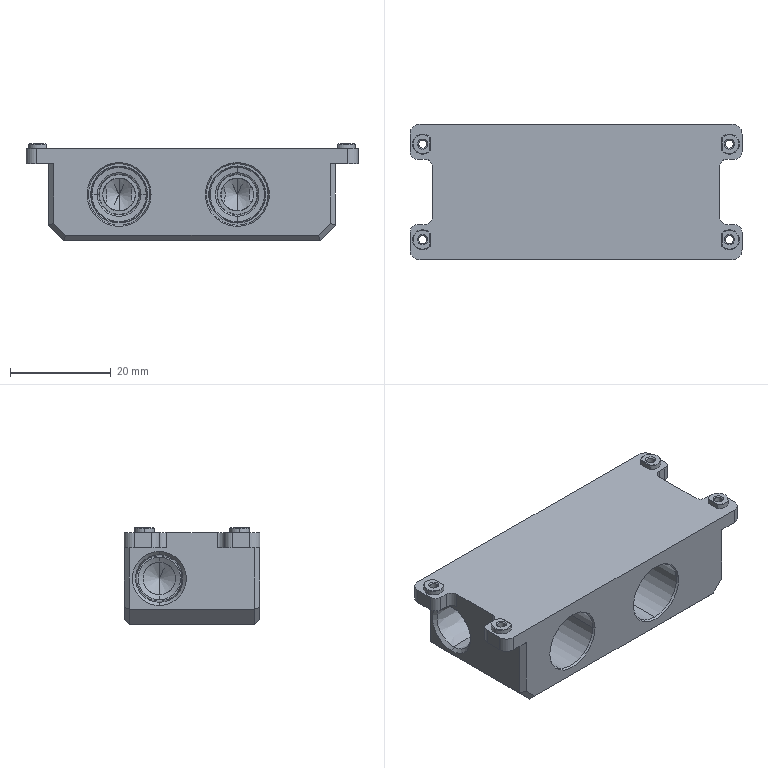NC program | NX | posted with a generic post | part box 66 x 27 x 19.25 mm
Lines 1 to 1685 of 6448, first 1517 of 1665 lines:
N10 G17 G21 G94 G90
(FLOOR_WALL , TOOL : D50面刀)
N12 T01 M6
N14 G53
N16 G17 G0 G90 X7.5 Y-69.5 S4500 M3
N18 G43 Z20. H1
N20 Z2.
N22 G94 G1 Z0. F800.
N24 Y-65.5
N26 Y65.5
N28 Y69.5
N30 Z2.
N32 G0 Z20.
N34 M5
(ADAPTIVE_MILLING , TOOL : D8开粗)
N36 T02 M6
N38 G53
N40 G17 G0 G90 X-7.067 Y-44.53 S7500 M3
N42 G43 Z20. H2
N44 Z-17.
N46 G94 G1 X-7.079 Y-44.38 Z-17.937 F2500.
N48 X-7.092 Y-44.231 Z-18.308
N50 X-7.105 Y-44.081 Z-18.58
N52 X-7.118 Y-43.932 Z-18.8
N54 X-7.131 Y-43.783 Z-18.984
N56 X-7.143 Y-43.633 Z-19.142
N58 X-7.156 Y-43.484 Z-19.28
N60 X-7.169 Y-43.334 Z-19.4
N62 X-7.182 Y-43.185 Z-19.505
N64 X-7.195 Y-43.035 Z-19.598
N66 X-7.207 Y-42.886 Z-19.679
N68 X-7.22 Y-42.736 Z-19.75
N70 X-7.233 Y-42.587 Z-19.81
N72 X-7.246 Y-42.437 Z-19.862
N74 X-7.259 Y-42.288 Z-19.905
N76 X-7.271 Y-42.139 Z-19.939
N78 X-7.284 Y-41.989 Z-19.966
N80 X-7.297 Y-41.84 Z-19.985
N82 X-7.31 Y-41.69 Z-19.996
N84 X-7.323 Y-41.541 Z-20.
N86 X-7.439 Y-40.185
N88 G3 X-7.858 Y-39.545 R0.809
N90 X-10.395 Y-38.825 R6.931
N92 X-13.916 Y-38.561 R62.132
N94 G2 X-16.854 Y-36.642 R4.621
N96 X-18.414 Y-32.843 R9.486
N98 X-18.931 Y-27.022 R34.366
N100 X-18.998 Y-14.123 R739.978
N102 G1 Y33.002
N104 G2 X-17.593 Y35.893 R4.169
N106 X-13.951 Y37.753 R8.174
N108 X-8.674 Y38.391 R25.798
N110 X4.375 Y38.498 R405.868
N112 G1 X13.774 Y38.484
N114 G2 X16.724 Y36.727 R4.45
N116 X18.401 Y32.833 R9.165
N118 X18.921 Y27.315 R32.513
N120 X18.998 Y13.965 R618.083
N122 G1 X18.996 Y-33.074
N124 G2 X17.436 Y-36.046 R4.252
N126 X13.741 Y-37.808 R8.515
N128 X8.383 Y-38.403 R27.886
N130 X-5.191 Y-38.477 R389.585
N132 X-9.5 Y-37.957 R98.771
N134 X-11.876 Y-37.672 R26.648
N136 X-14.578 Y-36.238 R6.14
N138 G1 X-14.89 Y-36.071
N140 X-15.814 Y-35.312
N142 X-16.573 Y-34.388
N144 X-17.136 Y-33.333
N146 X-17.483 Y-32.189
N148 G2 X-17.971 Y-22.311 R90.901
N150 G1 X-17.998 Y-11.361
N152 X-17.995 Y30.451
N154 G2 X-17.182 Y33.181 R5.655
N156 G1 X-17.135 Y33.336
N158 X-16.571 Y34.39
N160 X-15.812 Y35.314
N162 X-14.888 Y36.073
N164 X-13.833 Y36.636
N166 X-12.689 Y36.983
N168 G2 X-3.186 Y37.47 R89.967
N170 X11.198 Y37.482 R854.468
N172 X13.687 Y36.68 R5.673
N174 G1 X13.836 Y36.635
N176 X14.89 Y36.071
N178 X15.814 Y35.312
N180 X16.573 Y34.388
N182 X17.136 Y33.333
N184 X17.483 Y32.189
N186 G2 X17.973 Y22.011 R93.894
N188 G1 X17.998 Y11.211
N190 X17.994 Y-30.473
N192 G2 X17.181 Y-33.183 R5.661
N194 G1 X17.135 Y-33.336
N196 X16.571 Y-34.39
N198 X15.812 Y-35.314
N200 X14.888 Y-36.073
N202 X13.833 Y-36.636
N204 X12.689 Y-36.983
N206 G2 X3.186 Y-37.47 R89.76
N208 X-4.013 Y-37.453 R161.594
N210 X-8.025 Y-37.1 R101.274
N212 G1 X-11.501
N214 X-12.691 Y-36.982
N216 X-13.836 Y-36.635
N218 X-14.89 Y-36.071
N220 X-15.814 Y-35.312
N222 X-16.573 Y-34.388
N224 X-17.136 Y-33.333
N226 X-17.483 Y-32.189
N228 X-17.6 Y-30.999
N230 Y31.001
N232 X-17.482 Y32.191
N234 X-17.135 Y33.336
N236 X-16.571 Y34.39
N238 X-15.812 Y35.314
N240 X-14.888 Y36.073
N242 X-13.833 Y36.636
N244 X-12.689 Y36.983
N246 X-11.499 Y37.1
N248 X-7.999
N250 G2 X-6.217 Y36.844 R10.21
N252 G3 X-0.835 Y36.531 R41.818
N254 X5.498 Y36.515 R159.228
N256 X6.014 Y36.736 R3.667
N258 G2 X8.001 Y37.1 R6.513
N260 G1 X11.501
N262 X12.691 Y36.982
N264 X13.696 Y36.677
N266 X12.691 Y36.982
N268 X11.501 Y37.1
N270 X8.001
N272 G3 X6.014 Y36.736 R6.511
N274 G2 X3.976 Y36.143 R4.98
N276 X-4.811 Y36.15 R48.551
N278 G1 X-6.012 Y36.735
N280 X-6.806 Y36.957
N282 G2 X-4.63 Y35.963 R5.64
N284 G3 X-1.794 Y35.249 R8.388
N286 X3.699 Y35.265 R22.919
N288 X4.286 Y35.691 R1.168
N290 G1 X5.103 Y36.292
N292 X5.507 Y36.489
N294 G3 X3.925 Y35.315 R4.978
N296 G2 X1.942 Y34.752 R4.985
N298 X-3.594 Y35.122 R14.488
N300 X-4.284 Y35.689 R1.743
N302 G1 X-4.767 Y36.045
N304 G2 X-3.673 Y35.039 R5.141
N306 G3 X-1.437 Y34.121 R5.114
N308 X2.909 Y34.214 R9.441
N310 X3.306 Y34.511 R1.102
N312 G2 X4.002 Y35.389 R3.398
N314 G3 X3.178 Y34.325 R4.895
N316 G2 X1.424 Y33.644 R3.476
N318 X-3.021 Y34.236 R7.576
N320 X-3.589 Y34.95 R2.111
N322 G1 X-3.692 Y35.059
N324 G2 X-3.111 Y34.21 R6.402
N326 G3 X-1.161 Y33.134 R3.673
N328 X2.458 Y33.297 R5.928
N330 X2.879 Y33.709 R0.968
N332 G2 X3.244 Y34.415 R2.657
N334 G3 X2.787 Y33.504 R4.138
N336 G2 X1.45 Y32.767 R2.46
N338 X-2.649 Y33.424 R5.234
N340 X-3.039 Y34.098 R1.424
N342 G1 X-3.121 Y34.224
N344 G2 X-2.766 Y33.438 R5.334
N346 G3 X-1.68 Y32.604 R1.715
N348 G1 X1.779 Y32.612
N350 G3 X2.673 Y33.211 R1.013
N352 G1 X2.845 Y33.627
N354 G2 X2.348 Y32.776 R1.859
N356 X1.647 Y32.6 R1.117
N358 G1 X-1.872 Y32.608
N360 G2 X-2.786 Y33.487 R1.175
N362 G3 X-2.191 Y32.685 R1.281
N364 X-1.83 Y32.603 R3.588
N366 X-1.039 Y33.062 R0.801
N368 G1 X-0.792 Y33.804 Z-19.95
N370 X-0.559 Y34.551 Z-19.9
N372 X-0.43 Y34.968 F15000.
N374 X-0.287 Y35.38
N376 X-0.193 Y35.527
N378 X-0.07 Y35.652
N380 X0.729 Y36.296
N382 X1.535 Y36.931
N384 G2 X4.369 Y38.638 R15.893
N386 X6.671 Y39.42 R13.606
N388 X10.502 Y39.697 R10.132
N390 G1 X11.781 Y39.548
N392 X13.059 Y39.38
N394 G2 X18.414 Y35.931 R8.207
N396 G1 X20.089 Y33.489
N398 G2 X19.686 Y32.278 R0.8
N400 G1 X19.467 Y32.204
N402 X18.066 Y31.726 Z-19.995 F2500.
N404 X17.992 Y31.687 Z-20.
N406 G3 X17.6 Y30.999 R0.801
N408 G1 Y-31.001
N410 X17.482 Y-32.191
N412 X17.135 Y-33.336
N414 X16.571 Y-34.39
N416 X15.812 Y-35.314
N418 X14.888 Y-36.073
N420 X13.833 Y-36.636
N422 X12.689 Y-36.983
N424 X11.5 Y-37.1
N426 X7.999
N428 G2 X6.234 Y-36.847 R9.97
N430 G3 X0.564 Y-36.526 R42.919
N432 G2 X-5.051 Y-36.337 R88.056
N434 G1 X-5.321 Y-36.398
N436 G2 X-6.991 Y-37.008 R6.001
N438 G1 X-8.076 Y-37.1
N440 G3 X-5.186 Y-36.333 R5.83
N442 G2 X-2.94 Y-36.014 R8.254
N444 X4.756 Y-36.137 R58.568
N446 X5.1 Y-36.291 R1.779
N448 G3 X6.806 Y-36.957 R6.106
N450 G2 X4.741 Y-36.026 R5.134
N452 G3 X2.153 Y-35.288 R7.255
N454 X-3.636 Y-35.214 R23.492
N456 X-4.286 Y-35.691 R1.219
N458 G2 X-5.237 Y-36.358 R7.524
N460 G3 X-3.928 Y-35.311 R5.046
N462 G2 X-2.163 Y-34.754 R4.126
N464 X3.549 Y-35.103 R14.797
N466 X3.929 Y-35.311 R1.336
N468 G3 X4.767 Y-36.045 R3.381
N470 G2 X3.672 Y-35.038 R5.148
N472 G3 X1.442 Y-34.112 R5.084
N474 X-2.901 Y-34.194 R9.244
N476 X-3.29 Y-34.487 R1.126
N478 G2 X-3.95 Y-35.334 R3.283
N480 G3 X-3.163 Y-34.301 R4.918
N482 G2 X-1.364 Y-33.617 R3.519
N484 X2.967 Y-34.2 R7.695
N486 X3.266 Y-34.449 R2.09
N488 G3 X3.692 Y-35.059 R3.921
N490 G2 X3.103 Y-34.197 R6.503
N492 G3 X1.168 Y-33.125 R3.676
N494 X-2.454 Y-33.282 R5.842
N496 X-2.873 Y-33.694 R0.969
N498 G2 X-3.244 Y-34.415 R2.691
N500 G3 X-2.781 Y-33.489 R4.198
N502 G2 X-1.393 Y-32.741 R2.457
N504 X2.594 Y-33.38 R5.259
N506 X3.039 Y-34.098 R1.452
N508 G1 X3.12 Y-34.224
N510 G2 X2.766 Y-33.438 R5.334
N512 G3 X1.683 Y-32.603 R1.68
N514 G1 X-1.782 Y-32.612
N516 G3 X-2.673 Y-33.211 R1.001
N518 G1 X-2.816 Y-33.557
N520 G2 X-2.348 Y-32.776 R1.662
N522 X-1.572 Y-32.6 R1.208
N524 G1 X1.872 Y-32.608
N526 G2 X2.786 Y-33.487 R1.17
N528 G3 X2.191 Y-32.685 R1.281
N530 X1.83 Y-32.603 R3.588
N532 X0.959 Y-33.332 R0.808
N534 G1 X0.843 Y-34.556
N536 X0.829 Y-34.705 Z-19.996
N538 X0.815 Y-34.854 Z-19.985
N540 X0.8 Y-35.004 Z-19.966
N542 X0.786 Y-35.153 Z-19.939
N544 X0.772 Y-35.302 Z-19.905
N546 X0.758 Y-35.452 Z-19.862
N548 X0.744 Y-35.601 Z-19.81
N550 X0.73 Y-35.75 Z-19.75
N552 X0.715 Y-35.9 Z-19.679
N554 X0.701 Y-36.049 Z-19.598
N556 X0.687 Y-36.198 Z-19.505
N558 X0.673 Y-36.348 Z-19.4
N560 X0.659 Y-36.497 Z-19.28
N562 X0.645 Y-36.646 Z-19.142
N564 X0.63 Y-36.796 Z-18.984
N566 X0.616 Y-36.945 Z-18.8
N568 X0.602 Y-37.094 Z-18.58
N570 X0.588 Y-37.244 Z-18.308
N572 X0.574 Y-37.393 Z-17.937
N574 X0.56 Y-37.542 Z-17.
N576 G0 Z20.
N578 X22.505 Y-26.375
N580 Z-12.149
N582 G1 X22.358 Y-26.402 Z-13.086
N584 X22.21 Y-26.429 Z-13.457
N586 X22.062 Y-26.455 Z-13.729
N588 X21.915 Y-26.482 Z-13.949
N590 X21.767 Y-26.509 Z-14.133
N592 X21.62 Y-26.536 Z-14.291
N594 X21.472 Y-26.563 Z-14.429
N596 X21.325 Y-26.589 Z-14.549
N598 X21.177 Y-26.616 Z-14.654
N600 X21.029 Y-26.643 Z-14.747
N602 X20.882 Y-26.67 Z-14.828
N604 X20.734 Y-26.697 Z-14.899
N606 X20.587 Y-26.723 Z-14.959
N608 X20.439 Y-26.75 Z-15.011
N610 X20.291 Y-26.777 Z-15.054
N612 X20.144 Y-26.804 Z-15.088
N614 X19.996 Y-26.83 Z-15.115
N616 X19.849 Y-26.857 Z-15.134
N618 X19.701 Y-26.884 Z-15.145
N620 X19.554 Y-26.911 Z-15.149
N622 X18.228 Y-27.152
N624 G3 X17.571 Y-27.845 R0.808
N626 G2 X17.229 Y-29.239 R5.006
N628 X16.29 Y-31.976 R13.258
N630 X12.957 Y-34.873 R6.244
N632 X9.311 Y-35.645 R9.607
N634 X6.058 Y-34.437 R5.789
N636 G3 X3.833 Y-32.747 R88.653
N638 X3.412 Y-32.6 R1.291
N640 G1 X2.062
N642 X3.562
N644 G2 X4.986 Y-33.196 R4.552
N646 G3 X7.979 Y-34.421 R8.886
N648 X12.721 Y-33.777 R7.291
N650 X14.956 Y-31.761 R7.081
N652 X16.89 Y-29.806 R12.8
N654 G1 X17.262 Y-29.13
N656 G2 X16.399 Y-30.4 R4.758
N658 X14.762 Y-31.919 R14.41
N660 X12.561 Y-32.776 R8.172
N662 X7.384 Y-32.658 R9.197
N664 G1 X7.114 Y-32.6
N666 X3.514
N668 X12.936
N670 X13.494 Y-32.487
N672 G2 X14.277 Y-32.764 R0.809
N674 G1 X15.211 Y-33.893
N676 X15.306 Y-34.009 Z-15.145
N678 X15.402 Y-34.124 Z-15.134
N680 X15.498 Y-34.24 Z-15.115
N682 X15.593 Y-34.355 Z-15.088
N684 X15.689 Y-34.471 Z-15.054
N686 X15.784 Y-34.587 Z-15.011
N688 X15.88 Y-34.702 Z-14.959
N690 X15.976 Y-34.818 Z-14.899
N692 X16.071 Y-34.933 Z-14.828
N694 X16.167 Y-35.049 Z-14.747
N696 X16.262 Y-35.164 Z-14.654
N698 X16.358 Y-35.28 Z-14.549
N700 X16.454 Y-35.396 Z-14.429
N702 X16.549 Y-35.511 Z-14.291
N704 X16.645 Y-35.627 Z-14.133
N706 X16.74 Y-35.742 Z-13.949
N708 X16.836 Y-35.858 Z-13.729
N710 X16.932 Y-35.974 Z-13.457
N712 X17.027 Y-36.089 Z-13.086
N714 X17.123 Y-36.205 Z-12.149
N716 G0 Z20.
N718 X-0.202 Y-37.471
N720 Z-12.149
N722 G1 X-0.239 Y-37.326 Z-13.086
N724 X-0.277 Y-37.181 Z-13.457
N726 X-0.314 Y-37.036 Z-13.729
N728 X-0.351 Y-36.89 Z-13.949
N730 X-0.389 Y-36.745 Z-14.133
N732 X-0.426 Y-36.6 Z-14.291
N734 X-0.464 Y-36.455 Z-14.429
N736 X-0.501 Y-36.309 Z-14.549
N738 X-0.538 Y-36.164 Z-14.654
N740 X-0.576 Y-36.019 Z-14.747
N742 X-0.613 Y-35.873 Z-14.828
N744 X-0.65 Y-35.728 Z-14.899
N746 X-0.688 Y-35.583 Z-14.959
N748 X-0.725 Y-35.438 Z-15.011
N750 X-0.763 Y-35.292 Z-15.054
N752 X-0.8 Y-35.147 Z-15.088
N754 X-0.837 Y-35.002 Z-15.115
N756 X-0.875 Y-34.857 Z-15.134
N758 X-0.912 Y-34.711 Z-15.145
N760 X-0.949 Y-34.566 Z-15.149
N762 X-1.299 Y-33.207
N764 G3 X-2.073 Y-32.6 R0.808
N766 X-2.762 Y-32.969 R1.093
N768 G2 X-7.735 Y-35.514 R9.254
N770 X-11.233 Y-35.67 R9.05
N772 X-14.94 Y-32.874 R5.359
N774 X-15.687 Y-31.154 R13.369
N776 G3 X-16.4 Y-30.399 R5.785
N778 G2 X-17.567 Y-27.873 R4.138
N780 G3 X-16.4 Y-30.399 R4.142
N782 G2 X-14.72 Y-32.296 R15.805
N784 G3 X-9.948 Y-34.601 R6.782
N786 X-4.721 Y-33.303 R8.806
N788 G2 X-3.372 Y-32.621 R9.201
N790 X-2.034 Y-32.6 R12.607
N792 G3 X-4.023 Y-32.63 R18.908
N794 G2 X-6.887 Y-33.205 R80.074
N796 X-11.357 Y-32.632 R7.653
N798 G3 X-12.499 Y-32.6 R6.331
N800 G2 X-15.4 Y-31.399 R4.268
N802 G1 X-15.718 Y-31.08
N804 G3 X-14.07 Y-32.287 R4.998
N806 X-12.499 Y-32.6 R4.755
N808 G1 X-9.106 Y-32.642
N810 X-8.25 Y-32.6
N812 X-3.75
N814 X-11.175
N816 G3 X-11.98 Y-33.342 R0.808
N818 G1 X-12.079 Y-34.556
N820 X-12.091 Y-34.706 Z-15.145
N822 X-12.104 Y-34.855 Z-15.134
N824 X-12.116 Y-35.005 Z-15.115
N826 X-12.128 Y-35.154 Z-15.088
N828 X-12.14 Y-35.304 Z-15.054
N830 X-12.152 Y-35.453 Z-15.011
N832 X-12.165 Y-35.603 Z-14.959
N834 X-12.177 Y-35.752 Z-14.899
N836 X-12.189 Y-35.902 Z-14.828
N838 X-12.201 Y-36.051 Z-14.747
N840 X-12.213 Y-36.201 Z-14.654
N842 X-12.226 Y-36.35 Z-14.549
N844 X-12.238 Y-36.5 Z-14.429
N846 X-12.25 Y-36.649 Z-14.291
N848 X-12.262 Y-36.799 Z-14.133
N850 X-12.274 Y-36.948 Z-13.949
N852 X-12.287 Y-37.098 Z-13.729
N854 X-12.299 Y-37.247 Z-13.457
N856 X-12.311 Y-37.397 Z-13.086
N858 X-12.323 Y-37.546 Z-12.149
N860 G0 Z20.
N862 X-22.51 Y26.513
N864 Z-12.149
N866 G1 X-22.363 Y26.538 Z-13.086
N868 X-22.215 Y26.563 Z-13.457
N870 X-22.067 Y26.589 Z-13.729
N872 X-21.919 Y26.614 Z-13.949
N874 X-21.771 Y26.64 Z-14.133
N876 X-21.623 Y26.665 Z-14.291
N878 X-21.475 Y26.69 Z-14.429
N880 X-21.328 Y26.716 Z-14.549
N882 X-21.18 Y26.741 Z-14.654
N884 X-21.032 Y26.766 Z-14.747
N886 X-20.884 Y26.792 Z-14.828
N888 X-20.736 Y26.817 Z-14.899
N890 X-20.588 Y26.842 Z-14.959
N892 X-20.441 Y26.868 Z-15.011
N894 X-20.293 Y26.893 Z-15.054
N896 X-20.145 Y26.918 Z-15.088
N898 X-19.997 Y26.944 Z-15.115
N900 X-19.849 Y26.969 Z-15.134
N902 X-19.701 Y26.995 Z-15.145
N904 X-19.554 Y27.02 Z-15.149
N906 X-18.223 Y27.248
N908 G3 X-17.558 Y27.943 R0.808
N910 G2 X-17.262 Y29.13 R4.193
N912 X-16.413 Y31.743 R16.127
N914 X-12.918 Y34.894 R6.326
N916 X-9.12 Y35.64 R9.137
N918 X-5.964 Y34.372 R5.947
N920 G3 X-3.801 Y32.726 R59.109
N922 X-3.407 Y32.6 R1.538
N924 G1 X-2.057
N926 X-3.557
N928 G2 X-4.964 Y33.185 R4.429
N930 G3 X-7.959 Y34.42 R9.076
N932 X-12.834 Y33.717 R7.252
N934 X-14.961 Y31.759 R7.177
N936 X-16.89 Y29.806 R12.981
N938 G1 X-17.262 Y29.13
N940 G2 X-16.399 Y30.4 R4.758
N942 X-14.777 Y31.91 R14.674
N944 X-12.204 Y32.873 R8.575
N946 X-7.463 Y32.682 R9.13
N948 G1 X-7.098 Y32.6
N950 X-3.498
N952 X-12.499
N954 G3 X-14.068 Y32.288 R4.757
N956 G2 X-14.891 Y32.509 R0.809
N958 G1 X-15.858 Y33.539
N960 X-15.961 Y33.648 Z-15.145
N962 X-16.063 Y33.758 Z-15.134
N964 X-16.166 Y33.867 Z-15.115
N966 X-16.269 Y33.977 Z-15.088
N968 X-16.371 Y34.086 Z-15.054
N970 X-16.474 Y34.195 Z-15.011
N972 X-16.577 Y34.305 Z-14.959
N974 X-16.679 Y34.414 Z-14.899
N976 X-16.782 Y34.523 Z-14.828
N978 X-16.885 Y34.633 Z-14.747
N980 X-16.987 Y34.742 Z-14.654
N982 X-17.09 Y34.852 Z-14.549
N984 X-17.192 Y34.961 Z-14.429
N986 X-17.295 Y35.07 Z-14.291
N988 X-17.398 Y35.18 Z-14.133
N990 X-17.5 Y35.289 Z-13.949
N992 X-17.603 Y35.398 Z-13.729
N994 X-17.706 Y35.508 Z-13.457
N996 X-17.808 Y35.617 Z-13.086
N998 X-17.911 Y35.727 Z-12.149
N1000 G0 Z20.
N1002 X0.192 Y37.47
N1004 Z-12.149
N1006 G1 X0.23 Y37.325 Z-13.086
N1008 X0.268 Y37.179 Z-13.457
N1010 X0.305 Y37.034 Z-13.729
N1012 X0.343 Y36.889 Z-13.949
N1014 X0.381 Y36.744 Z-14.133
N1016 X0.418 Y36.599 Z-14.291
N1018 X0.456 Y36.453 Z-14.429
N1020 X0.494 Y36.308 Z-14.549
N1022 X0.532 Y36.163 Z-14.654
N1024 X0.569 Y36.018 Z-14.747
N1026 X0.607 Y35.873 Z-14.828
N1028 X0.645 Y35.728 Z-14.899
N1030 X0.682 Y35.582 Z-14.959
N1032 X0.72 Y35.437 Z-15.011
N1034 X0.758 Y35.292 Z-15.054
N1036 X0.795 Y35.147 Z-15.088
N1038 X0.833 Y35.002 Z-15.115
N1040 X0.871 Y34.856 Z-15.134
N1042 X0.909 Y34.711 Z-15.145
N1044 X0.946 Y34.566 Z-15.149
N1046 X1.3 Y33.205
N1048 G3 X2.073 Y32.6 R0.808
N1050 X2.708 Y32.927 R1.003
N1052 G2 X5.304 Y34.759 R9.718
N1054 X10.488 Y35.768 R11.963
N1056 X14.976 Y32.815 R5.391
N1058 X15.687 Y31.158 R13.902
N1060 G3 X16.4 Y30.399 R5.806
N1062 G2 X17.567 Y27.873 R4.138
N1064 G3 X16.4 Y30.399 R4.142
N1066 G2 X14.701 Y32.322 R17.267
N1068 G3 X9.815 Y34.615 R6.815
N1070 X4.802 Y33.352 R8.754
N1072 G2 X3.342 Y32.615 R8.062
N1074 G1 X2.038 Y32.6
N1076 G3 X4.014 Y32.629 R19.213
N1078 G2 X6.825 Y33.199 R89.925
N1080 X11.368 Y32.632 R7.664
N1082 G3 X12.501 Y32.6 R6.265
N1084 G2 X15.678 Y31.132 R4.34
N1086 G3 X12.501 Y32.6 R4.323
N1088 G2 X9.133 Y32.645 R359.237
N1090 G1 X8.216 Y32.6
N1092 X3.716
N1094 X11.216
N1096 G3 X12.021 Y33.337 R0.808
N1098 G1 X12.128 Y34.556
N1100 X12.142 Y34.705 Z-15.145
N1102 X12.155 Y34.855 Z-15.134
N1104 X12.168 Y35.004 Z-15.115
N1106 X12.181 Y35.154 Z-15.088
N1108 X12.194 Y35.303 Z-15.054
N1110 X12.207 Y35.453 Z-15.011
N1112 X12.221 Y35.602 Z-14.959
N1114 X12.234 Y35.751 Z-14.899
N1116 X12.247 Y35.901 Z-14.828
N1118 X12.26 Y36.05 Z-14.747
N1120 X12.273 Y36.2 Z-14.654
N1122 X12.286 Y36.349 Z-14.549
N1124 X12.3 Y36.499 Z-14.429
N1126 X12.313 Y36.648 Z-14.291
N1128 X12.326 Y36.797 Z-14.133
N1130 X12.339 Y36.947 Z-13.949
N1132 X12.352 Y37.096 Z-13.729
N1134 X12.366 Y37.246 Z-13.457
N1136 X12.379 Y37.395 Z-13.086
N1138 X12.392 Y37.544 Z-12.149
N1140 G0 Z20.
N1142 X22.493 Y-25.889
N1144 Z0.
N1146 G1 X22.346 Y-25.92 Z-0.937
N1148 X22.199 Y-25.951 Z-1.308
N1150 X22.052 Y-25.981 Z-1.58
N1152 X21.905 Y-26.012 Z-1.8
N1154 X21.758 Y-26.042 Z-1.984
N1156 X21.612 Y-26.073 Z-2.142
N1158 X21.465 Y-26.103 Z-2.28
N1160 X21.318 Y-26.134 Z-2.4
N1162 X21.171 Y-26.165 Z-2.505
N1164 X21.024 Y-26.195 Z-2.598
N1166 X20.877 Y-26.226 Z-2.679
N1168 X20.731 Y-26.256 Z-2.75
N1170 X20.584 Y-26.287 Z-2.81
N1172 X20.437 Y-26.318 Z-2.862
N1174 X20.29 Y-26.348 Z-2.905
N1176 X20.143 Y-26.379 Z-2.939
N1178 X19.996 Y-26.409 Z-2.966
N1180 X19.849 Y-26.44 Z-2.985
N1182 X19.703 Y-26.47 Z-2.996
N1184 X19.556 Y-26.501 Z-3.
N1186 X18.194 Y-26.785
N1188 G3 X17.556 Y-27.487 R0.809
N1190 G2 X17.248 Y-28.749 R4.366
N1192 X15.711 Y-31.028 R12.796
N1194 G3 X15.582 Y-31.866 R0.809
N1196 G1 X16.176 Y-33.278
N1198 X16.234 Y-33.416 Z-2.996
N1200 X16.293 Y-33.554 Z-2.985
N1202 X16.351 Y-33.693 Z-2.966
N1204 X16.409 Y-33.831 Z-2.939
N1206 X16.467 Y-33.969 Z-2.905
N1208 X16.525 Y-34.107 Z-2.862
N1210 X16.584 Y-34.246 Z-2.81
N1212 X16.642 Y-34.384 Z-2.75
N1214 X16.7 Y-34.522 Z-2.679
N1216 X16.758 Y-34.66 Z-2.598
N1218 X16.817 Y-34.799 Z-2.505
N1220 X16.875 Y-34.937 Z-2.4
N1222 X16.933 Y-35.075 Z-2.28
N1224 X16.991 Y-35.213 Z-2.142
N1226 X17.049 Y-35.352 Z-1.984
N1228 X17.108 Y-35.49 Z-1.8
N1230 X17.166 Y-35.628 Z-1.58
N1232 X17.224 Y-35.766 Z-1.308
N1234 X17.282 Y-35.905 Z-0.937
N1236 X17.34 Y-36.043 Z0.
N1238 G0 Z20.
N1240 X-17.886 Y-35.759
N1242 Z0.
N1244 G1 X-17.8 Y-35.637 Z-0.937
N1246 X-17.713 Y-35.514 Z-1.308
N1248 X-17.626 Y-35.392 Z-1.58
N1250 X-17.54 Y-35.269 Z-1.8
N1252 X-17.453 Y-35.147 Z-1.984
N1254 X-17.366 Y-35.024 Z-2.142
N1256 X-17.28 Y-34.902 Z-2.28
N1258 X-17.193 Y-34.78 Z-2.4
N1260 X-17.106 Y-34.657 Z-2.505
N1262 X-17.02 Y-34.535 Z-2.598
N1264 X-16.933 Y-34.412 Z-2.679
N1266 X-16.846 Y-34.29 Z-2.75
N1268 X-16.76 Y-34.167 Z-2.81
N1270 X-16.673 Y-34.045 Z-2.862
N1272 X-16.586 Y-33.923 Z-2.905
N1274 X-16.5 Y-33.8 Z-2.939
N1276 X-16.413 Y-33.678 Z-2.966
N1278 X-16.326 Y-33.555 Z-2.985
N1280 X-16.24 Y-33.433 Z-2.996
N1282 X-16.153 Y-33.31 Z-3.
N1284 X-15.435 Y-32.295
N1286 G3 X-15.477 Y-31.307 R0.808
N1288 G2 X-17.249 Y-28.746 R13.167
N1290 X-17.556 Y-27.485 R4.37
N1292 G3 X-18.194 Y-26.783 R0.809
N1294 G1 X-19.556 Y-26.499
N1296 X-19.703 Y-26.468 Z-2.996
N1298 X-19.849 Y-26.438 Z-2.985
N1300 X-19.996 Y-26.407 Z-2.966
N1302 X-20.143 Y-26.377 Z-2.939
N1304 X-20.29 Y-26.346 Z-2.905
N1306 X-20.437 Y-26.315 Z-2.862
N1308 X-20.584 Y-26.285 Z-2.81
N1310 X-20.731 Y-26.254 Z-2.75
N1312 X-20.877 Y-26.223 Z-2.679
N1314 X-21.024 Y-26.193 Z-2.598
N1316 X-21.171 Y-26.162 Z-2.505
N1318 X-21.318 Y-26.132 Z-2.4
N1320 X-21.465 Y-26.101 Z-2.28
N1322 X-21.612 Y-26.07 Z-2.142
N1324 X-21.758 Y-26.04 Z-1.984
N1326 X-21.905 Y-26.009 Z-1.8
N1328 X-22.052 Y-25.979 Z-1.58
N1330 X-22.199 Y-25.948 Z-1.308
N1332 X-22.346 Y-25.917 Z-0.937
N1334 X-22.493 Y-25.887 Z0.
N1336 G0 Z20.
N1338 X22.495 Y-25.355
N1340 Z0.5
N1342 G1 X22.348 Y-25.385 Z-0.437
N1344 X22.201 Y-25.415 Z-0.808
N1346 X22.054 Y-25.445 Z-1.08
N1348 X21.907 Y-25.475 Z-1.3
N1350 X21.76 Y-25.505 Z-1.484
N1352 X21.613 Y-25.535 Z-1.642
N1354 X21.466 Y-25.565 Z-1.78
N1356 X21.319 Y-25.595 Z-1.9
N1358 X21.172 Y-25.626 Z-2.005
N1360 X21.025 Y-25.656 Z-2.098
N1362 X20.878 Y-25.686 Z-2.179
N1364 X20.731 Y-25.716 Z-2.25
N1366 X20.584 Y-25.746 Z-2.31
N1368 X20.437 Y-25.776 Z-2.362
N1370 X20.291 Y-25.806 Z-2.405
N1372 X20.144 Y-25.836 Z-2.439
N1374 X19.997 Y-25.866 Z-2.466
N1376 X19.85 Y-25.896 Z-2.485
N1378 X19.703 Y-25.927 Z-2.496
N1380 X19.556 Y-25.957 Z-2.5
N1382 X18.202 Y-26.234
N1384 G3 X17.559 Y-26.95 R0.808
N1386 G1 X17.518 Y-27.39
N1388 G2 X16.836 Y-28.996 R4.972
N1390 G1 X15.836 Y-30.41
N1392 X15.184 Y-31.133
N1394 X14.379 Y-31.682
N1396 X13.467 Y-32.024
N1398 X12.5 Y-32.141
N1400 X-12.501
N1402 X-13.467 Y-32.024
N1404 X-14.379 Y-31.682
N1406 X-15.184 Y-31.133
N1408 G2 X-17.26 Y-28.228 R13.268
N1410 G1 X-17.518 Y-27.391
N1412 X-17.546 Y-27.092
N1414 G3 X-18.2 Y-26.374 R0.808
N1416 G1 X-19.556 Y-26.117
N1418 X-19.703 Y-26.089 Z-2.496
N1420 X-19.851 Y-26.061 Z-2.485
N1422 X-19.998 Y-26.033 Z-2.466
N1424 X-20.145 Y-26.005 Z-2.439
N1426 X-20.293 Y-25.977 Z-2.405
N1428 X-20.44 Y-25.949 Z-2.362
N1430 X-20.587 Y-25.921 Z-2.31
N1432 X-20.735 Y-25.894 Z-2.25
N1434 X-20.882 Y-25.866 Z-2.179
N1436 X-21.03 Y-25.838 Z-2.098
N1438 X-21.177 Y-25.81 Z-2.005
N1440 X-21.324 Y-25.782 Z-1.9
N1442 X-21.472 Y-25.754 Z-1.78
N1444 X-21.619 Y-25.726 Z-1.642
N1446 X-21.766 Y-25.698 Z-1.484
N1448 X-21.914 Y-25.67 Z-1.3
N1450 X-22.061 Y-25.642 Z-1.08
N1452 X-22.209 Y-25.614 Z-0.808
N1454 X-22.356 Y-25.586 Z-0.437
N1456 X-22.503 Y-25.558 Z0.5
N1458 G0 Z20.
N1460 X22.49 Y-24.84
N1462 Z1.
N1464 G1 X22.343 Y-24.871 Z0.063
N1466 X22.196 Y-24.902 Z-0.308
N1468 X22.05 Y-24.933 Z-0.58
N1470 X21.903 Y-24.965 Z-0.8
N1472 X21.756 Y-24.996 Z-0.984
N1474 X21.61 Y-25.027 Z-1.142
N1476 X21.463 Y-25.058 Z-1.28
N1478 X21.316 Y-25.09 Z-1.4
N1480 X21.169 Y-25.121 Z-1.505
N1482 X21.023 Y-25.152 Z-1.598
N1484 X20.876 Y-25.184 Z-1.679
N1486 X20.729 Y-25.215 Z-1.75
N1488 X20.583 Y-25.246 Z-1.81
N1490 X20.436 Y-25.277 Z-1.862
N1492 X20.289 Y-25.309 Z-1.905
N1494 X20.143 Y-25.34 Z-1.939
N1496 X19.996 Y-25.371 Z-1.966
N1498 X19.849 Y-25.403 Z-1.985
N1500 X19.702 Y-25.434 Z-1.996
N1502 X19.556 Y-25.465 Z-2.
N1504 X18.194 Y-25.755
N1506 G3 X17.559 Y-26.458 R0.809
N1508 G2 X17.249 Y-27.749 R4.37
N1510 X15.184 Y-30.633 R13.285
N1512 G1 X14.379 Y-31.182
N1514 X13.467 Y-31.524
N1516 X12.5 Y-31.641
N1518 X-12.501
N1520 X-13.467 Y-31.524
N1522 X-14.379 Y-31.182
N1524 X-15.184 Y-30.633
N1526 G2 X-17.25 Y-27.747 R13.278
N1528 X-17.556 Y-26.486 R4.341
N1530 G3 X-18.194 Y-25.782 R0.809
N1532 G1 X-19.556 Y-25.497
N1534 X-19.703 Y-25.466 Z-1.996
N1536 X-19.849 Y-25.435 Z-1.985
N1538 X-19.996 Y-25.404 Z-1.966
N1540 X-20.143 Y-25.373 Z-1.939
N1542 X-20.29 Y-25.343 Z-1.905
N1544 X-20.437 Y-25.312 Z-1.862
N1546 X-20.583 Y-25.281 Z-1.81
N1548 X-20.73 Y-25.25 Z-1.75
N1550 X-20.877 Y-25.219 Z-1.679
N1552 X-21.024 Y-25.189 Z-1.598
N1554 X-21.171 Y-25.158 Z-1.505
N1556 X-21.317 Y-25.127 Z-1.4
N1558 X-21.464 Y-25.096 Z-1.28
N1560 X-21.611 Y-25.066 Z-1.142
N1562 X-21.758 Y-25.035 Z-0.984
N1564 X-21.905 Y-25.004 Z-0.8
N1566 X-22.052 Y-24.973 Z-0.58
N1568 X-22.198 Y-24.942 Z-0.308
N1570 X-22.345 Y-24.912 Z0.063
N1572 X-22.492 Y-24.881 Z1.
N1574 G0 Z20.
N1576 X22.482 Y-24.205
N1578 Z1.5
N1580 G1 X22.336 Y-24.238 Z0.563
N1582 X22.19 Y-24.271 Z0.192
N1584 X22.043 Y-24.304 Z-0.08
N1586 X21.897 Y-24.337 Z-0.3
N1588 X21.751 Y-24.37 Z-0.484
N1590 X21.604 Y-24.403 Z-0.642
N1592 X21.458 Y-24.436 Z-0.78
N1594 X21.312 Y-24.469 Z-0.9
N1596 X21.165 Y-24.502 Z-1.005
N1598 X21.019 Y-24.535 Z-1.098
N1600 X20.873 Y-24.568 Z-1.179
N1602 X20.726 Y-24.601 Z-1.25
N1604 X20.58 Y-24.634 Z-1.31
N1606 X20.434 Y-24.667 Z-1.362
N1608 X20.287 Y-24.7 Z-1.405
N1610 X20.141 Y-24.733 Z-1.439
N1612 X19.995 Y-24.766 Z-1.466
N1614 X19.848 Y-24.799 Z-1.485
N1616 X19.702 Y-24.832 Z-1.496
N1618 X19.556 Y-24.864 Z-1.5
N1620 X18.193 Y-25.171
N1622 G3 X17.568 Y-25.869 R0.809
N1624 G2 X17.246 Y-27.248 R4.569
N1626 X15.184 Y-30.133 R13.14
N1628 G1 X14.379 Y-30.682
N1630 X13.467 Y-31.024
N1632 X12.5 Y-31.141
N1634 X-12.501
N1636 X-13.467 Y-31.024
N1638 X-14.379 Y-30.682
N1640 X-15.184 Y-30.133
N1642 G2 X-17.252 Y-27.247 R13.353
N1644 X-17.549 Y-26.06 R4.255
N1646 G3 X-18.194 Y-25.354 R0.808
N1648 G1 X-19.556 Y-25.081
N1650 X-19.703 Y-25.052 Z-1.496
N1652 X-19.85 Y-25.022 Z-1.485
N1654 X-19.997 Y-24.993 Z-1.466
N1656 X-20.144 Y-24.963 Z-1.439
N1658 X-20.291 Y-24.934 Z-1.405
N1660 X-20.438 Y-24.904 Z-1.362
N1662 X-20.585 Y-24.875 Z-1.31
N1664 X-20.732 Y-24.845 Z-1.25
N1666 X-20.879 Y-24.816 Z-1.179
N1668 X-21.027 Y-24.786 Z-1.098
N1670 X-21.174 Y-24.757 Z-1.005
N1672 X-21.321 Y-24.728 Z-0.9
N1674 X-21.468 Y-24.698 Z-0.78
N1676 X-21.615 Y-24.669 Z-0.642
N1678 X-21.762 Y-24.639 Z-0.484
N1680 X-21.909 Y-24.61 Z-0.3
N1682 X-22.056 Y-24.58 Z-0.08
N1684 X-22.203 Y-24.551 Z0.192
N1686 X-22.35 Y-24.521 Z0.563
N1688 X-22.497 Y-24.492 Z1.5
N1690 G0 Z20.
N1692 X22.52 Y-25.293
N1694 Z2.
N1696 G1 X22.371 Y-25.274 Z1.063
N1698 X22.222 Y-25.255 Z0.692
N1700 X22.073 Y-25.236 Z0.42
N1702 X21.925 Y-25.217 Z0.2
N1704 X21.776 Y-25.198 Z0.016
N1706 X21.627 Y-25.179 Z-0.142
N1708 X21.478 Y-25.16 Z-0.28
N1710 X21.329 Y-25.141 Z-0.4
N1712 X21.181 Y-25.122 Z-0.505
N1714 X21.032 Y-25.103 Z-0.598
N1716 X20.883 Y-25.084 Z-0.679
N1718 X20.734 Y-25.065 Z-0.75
N1720 X20.586 Y-25.046 Z-0.81
N1722 X20.437 Y-25.027 Z-0.862
N1724 X20.288 Y-25.008 Z-0.905
N1726 X20.139 Y-24.989 Z-0.939
N1728 X19.99 Y-24.97 Z-0.966
N1730 X19.842 Y-24.951 Z-0.985
N1732 X19.693 Y-24.932 Z-0.996
N1734 X19.544 Y-24.913 Z-1.
N1736 X18.461 Y-24.775
N1738 G3 X17.557 Y-25.471 R0.808
N1740 G2 X16.839 Y-27.493 R4.183
N1742 G1 X15.836 Y-28.91
N1744 X15.184 Y-29.633
N1746 X14.379 Y-30.182
N1748 X13.467 Y-30.524
N1750 X12.5 Y-30.641
N1752 X-12.501
N1754 X-13.467 Y-30.524
N1756 X-14.379 Y-30.182
N1758 X-15.184 Y-29.633
N1760 G2 X-17.199 Y-26.85 R13.463
N1762 X-17.561 Y-25.565 R4.429
N1764 G3 X-18.156 Y-24.93 R0.809
N1766 G1 X-19.542 Y-24.578
N1768 X-19.687 Y-24.541 Z-0.996
N1770 X-19.833 Y-24.504 Z-0.985
N1772 X-19.978 Y-24.467 Z-0.966
N1774 X-20.124 Y-24.431 Z-0.939
N1776 X-20.269 Y-24.394 Z-0.905
N1778 X-20.414 Y-24.357 Z-0.862
N1780 X-20.56 Y-24.32 Z-0.81
N1782 X-20.705 Y-24.283 Z-0.75
N1784 X-20.851 Y-24.246 Z-0.679
N1786 X-20.996 Y-24.209 Z-0.598
N1788 X-21.141 Y-24.172 Z-0.505
N1790 X-21.287 Y-24.136 Z-0.4
N1792 X-21.432 Y-24.099 Z-0.28
N1794 X-21.578 Y-24.062 Z-0.142
N1796 X-21.723 Y-24.025 Z0.016
N1798 X-21.868 Y-23.988 Z0.2
N1800 X-22.014 Y-23.951 Z0.42
N1802 X-22.159 Y-23.914 Z0.692
N1804 X-22.304 Y-23.877 Z1.063
N1806 X-22.45 Y-23.841 Z2.
N1808 G0 Z20.
N1810 X-22.495 Y25.925
N1812 Z0.
N1814 G1 X-22.348 Y25.955 Z-0.937
N1816 X-22.201 Y25.985 Z-1.308
N1818 X-22.054 Y26.015 Z-1.58
N1820 X-21.907 Y26.045 Z-1.8
N1822 X-21.76 Y26.075 Z-1.984
N1824 X-21.613 Y26.105 Z-2.142
N1826 X-21.466 Y26.135 Z-2.28
N1828 X-21.319 Y26.166 Z-2.4
N1830 X-21.172 Y26.196 Z-2.505
N1832 X-21.025 Y26.226 Z-2.598
N1834 X-20.878 Y26.256 Z-2.679
N1836 X-20.731 Y26.286 Z-2.75
N1838 X-20.584 Y26.316 Z-2.81
N1840 X-20.437 Y26.346 Z-2.862
N1842 X-20.291 Y26.376 Z-2.905
N1844 X-20.144 Y26.406 Z-2.939
N1846 X-19.997 Y26.436 Z-2.966
N1848 X-19.85 Y26.466 Z-2.985
N1850 X-19.703 Y26.496 Z-2.996
N1852 X-19.556 Y26.526 Z-3.
N1854 X-18.196 Y26.804
N1856 G3 X-17.554 Y27.51 R0.808
N1858 G2 X-17.251 Y28.75 R4.275
N1860 X-15.473 Y31.312 R13.477
N1862 G3 X-15.429 Y32.299 R0.808
N1864 G1 X-16.146 Y33.316
N1866 X-16.232 Y33.439 Z-2.996
N1868 X-16.319 Y33.561 Z-2.985
N1870 X-16.405 Y33.684 Z-2.966
N1872 X-16.491 Y33.807 Z-2.939
N1874 X-16.578 Y33.929 Z-2.905
N1876 X-16.664 Y34.052 Z-2.862
N1878 X-16.751 Y34.174 Z-2.81
N1880 X-16.837 Y34.297 Z-2.75
N1882 X-16.923 Y34.42 Z-2.679
N1884 X-17.01 Y34.542 Z-2.598
N1886 X-17.096 Y34.665 Z-2.505
N1888 X-17.183 Y34.788 Z-2.4
N1890 X-17.269 Y34.91 Z-2.28
N1892 X-17.356 Y35.033 Z-2.142
N1894 X-17.442 Y35.155 Z-1.984
N1896 X-17.528 Y35.278 Z-1.8
N1898 X-17.615 Y35.401 Z-1.58
N1900 X-17.701 Y35.523 Z-1.308
N1902 X-17.788 Y35.646 Z-0.937
N1904 X-17.874 Y35.768 Z0.
N1906 G0 Z20.
N1908 X18.716 Y35.076
N1910 Z0.
N1912 G1 X18.616 Y34.964 Z-0.937
N1914 X18.516 Y34.853 Z-1.308
N1916 X18.416 Y34.741 Z-1.58
N1918 X18.316 Y34.629 Z-1.8
N1920 X18.216 Y34.517 Z-1.984
N1922 X18.116 Y34.406 Z-2.142
N1924 X18.016 Y34.294 Z-2.28
N1926 X17.916 Y34.182 Z-2.4
N1928 X17.815 Y34.071 Z-2.505
N1930 X17.715 Y33.959 Z-2.598
N1932 X17.615 Y33.847 Z-2.679
N1934 X17.515 Y33.735 Z-2.75
N1936 X17.415 Y33.624 Z-2.81
N1938 X17.315 Y33.512 Z-2.862
N1940 X17.215 Y33.4 Z-2.905
N1942 X17.115 Y33.289 Z-2.939
N1944 X17.015 Y33.177 Z-2.966
N1946 X16.915 Y33.065 Z-2.985
N1948 X16.815 Y32.953 Z-2.996
N1950 X16.714 Y32.842 Z-3.
N1952 X15.89 Y31.921
N1954 G3 X15.832 Y30.916 R0.808
N1956 G1 X16.837 Y29.494
N1958 G2 X17.509 Y27.933 R4.96
N1960 G1 X17.557 Y27.486
N1962 G3 X18.192 Y26.782 R0.809
N1964 G1 X19.556 Y26.49
N1966 X19.702 Y26.459 Z-2.996
N1968 X19.849 Y26.428 Z-2.985
N1970 X19.996 Y26.396 Z-2.966
N1972 X20.143 Y26.365 Z-2.939
N1974 X20.289 Y26.334 Z-2.905
N1976 X20.436 Y26.302 Z-2.862
N1978 X20.583 Y26.271 Z-2.81
N1980 X20.729 Y26.24 Z-2.75
N1982 X20.876 Y26.208 Z-2.679
N1984 X21.023 Y26.177 Z-2.598
N1986 X21.169 Y26.146 Z-2.505
N1988 X21.316 Y26.114 Z-2.4
N1990 X21.463 Y26.083 Z-2.28
N1992 X21.609 Y26.052 Z-2.142
N1994 X21.756 Y26.02 Z-1.984
N1996 X21.903 Y25.989 Z-1.8
N1998 X22.05 Y25.958 Z-1.58
N2000 X22.196 Y25.926 Z-1.308
N2002 X22.343 Y25.895 Z-0.937
N2004 X22.49 Y25.864 Z0.
N2006 G0 Z20.
N2008 X-22.495 Y25.355
N2010 Z0.5
N2012 G1 X-22.348 Y25.385 Z-0.437
N2014 X-22.201 Y25.415 Z-0.808
N2016 X-22.054 Y25.445 Z-1.08
N2018 X-21.907 Y25.475 Z-1.3
N2020 X-21.76 Y25.505 Z-1.484
N2022 X-21.613 Y25.535 Z-1.642
N2024 X-21.466 Y25.565 Z-1.78
N2026 X-21.319 Y25.595 Z-1.9
N2028 X-21.172 Y25.625 Z-2.005
N2030 X-21.025 Y25.655 Z-2.098
N2032 X-20.878 Y25.685 Z-2.179
N2034 X-20.731 Y25.715 Z-2.25
N2036 X-20.585 Y25.745 Z-2.31
N2038 X-20.438 Y25.775 Z-2.362
N2040 X-20.291 Y25.805 Z-2.405
N2042 X-20.144 Y25.835 Z-2.439
N2044 X-19.997 Y25.865 Z-2.466
N2046 X-19.85 Y25.895 Z-2.485
N2048 X-19.703 Y25.925 Z-2.496
N2050 X-19.556 Y25.955 Z-2.5
N2052 X-18.202 Y26.232
N2054 G3 X-17.56 Y26.948 R0.808
N2056 G1 X-17.518 Y27.391
N2058 G2 X-16.836 Y28.996 R4.97
N2060 G1 X-15.866 Y30.367
N2062 X-15.21 Y31.105
N2064 X-14.398 Y31.665
N2066 X-13.478 Y32.017
N2068 X-12.499 Y32.141
N2070 X12.501
N2072 X13.467 Y32.024
N2074 X14.379 Y31.682
N2076 X15.184 Y31.133
N2078 G2 X17.26 Y28.228 R13.262
N2080 G1 X17.518 Y27.39
N2082 X17.553 Y27.016
N2084 G3 X18.201 Y26.299 R0.808
N2086 G1 X19.556 Y26.032
N2088 X19.703 Y26.003 Z-2.496
N2090 X19.85 Y25.974 Z-2.485
N2092 X19.997 Y25.945 Z-2.466
N2094 X20.144 Y25.915 Z-2.439
N2096 X20.292 Y25.886 Z-2.405
N2098 X20.439 Y25.857 Z-2.362
N2100 X20.586 Y25.828 Z-2.31
N2102 X20.733 Y25.799 Z-2.25
N2104 X20.88 Y25.77 Z-2.179
N2106 X21.027 Y25.741 Z-2.098
N2108 X21.175 Y25.712 Z-2.005
N2110 X21.322 Y25.683 Z-1.9
N2112 X21.469 Y25.654 Z-1.78
N2114 X21.616 Y25.625 Z-1.642
N2116 X21.763 Y25.596 Z-1.484
N2118 X21.91 Y25.567 Z-1.3
N2120 X22.058 Y25.538 Z-1.08
N2122 X22.205 Y25.509 Z-0.808
N2124 X22.352 Y25.48 Z-0.437
N2126 X22.499 Y25.451 Z0.5
N2128 G0 Z20.
N2130 X-22.49 Y24.838
N2132 Z1.
N2134 G1 X-22.343 Y24.87 Z0.063
N2136 X-22.196 Y24.901 Z-0.308
N2138 X-22.05 Y24.932 Z-0.58
N2140 X-21.903 Y24.963 Z-0.8
N2142 X-21.756 Y24.995 Z-0.984
N2144 X-21.61 Y25.026 Z-1.142
N2146 X-21.463 Y25.057 Z-1.28
N2148 X-21.316 Y25.089 Z-1.4
N2150 X-21.169 Y25.12 Z-1.505
N2152 X-21.023 Y25.151 Z-1.598
N2154 X-20.876 Y25.182 Z-1.679
N2156 X-20.729 Y25.214 Z-1.75
N2158 X-20.583 Y25.245 Z-1.81
N2160 X-20.436 Y25.276 Z-1.862
N2162 X-20.289 Y25.308 Z-1.905
N2164 X-20.143 Y25.339 Z-1.939
N2166 X-19.996 Y25.37 Z-1.966
N2168 X-19.849 Y25.401 Z-1.985
N2170 X-19.702 Y25.433 Z-1.996
N2172 X-19.556 Y25.464 Z-2.
N2174 X-18.194 Y25.754
N2176 G3 X-17.559 Y26.457 R0.809
N2178 G2 X-17.249 Y27.749 R4.369
N2180 X-15.184 Y30.633 R13.289
N2182 G1 X-14.379 Y31.182
N2184 X-13.467 Y31.524
N2186 X-12.499 Y31.641
N2188 X12.501
N2190 X13.467 Y31.524
N2192 X14.379 Y31.182
N2194 X15.184 Y30.633
N2196 G2 X17.25 Y27.747 R13.274
N2198 X17.556 Y26.486 R4.343
N2200 G3 X18.194 Y25.782 R0.809
N2202 G1 X19.556 Y25.497
N2204 X19.703 Y25.466 Z-1.996
N2206 X19.849 Y25.435 Z-1.985
N2208 X19.996 Y25.404 Z-1.966
N2210 X20.143 Y25.373 Z-1.939
N2212 X20.29 Y25.343 Z-1.905
N2214 X20.437 Y25.312 Z-1.862
N2216 X20.583 Y25.281 Z-1.81
N2218 X20.73 Y25.25 Z-1.75
N2220 X20.877 Y25.219 Z-1.679
N2222 X21.024 Y25.189 Z-1.598
N2224 X21.171 Y25.158 Z-1.505
N2226 X21.317 Y25.127 Z-1.4
N2228 X21.464 Y25.096 Z-1.28
N2230 X21.611 Y25.065 Z-1.142
N2232 X21.758 Y25.035 Z-0.984
N2234 X21.905 Y25.004 Z-0.8
N2236 X22.051 Y24.973 Z-0.58
N2238 X22.198 Y24.942 Z-0.308
N2240 X22.345 Y24.911 Z0.063
N2242 X22.492 Y24.881 Z1.
N2244 G0 Z20.
N2246 X-22.491 Y24.349
N2248 Z1.5
N2250 G1 X-22.344 Y24.38 Z0.563
N2252 X-22.197 Y24.411 Z0.192
N2254 X-22.05 Y24.442 Z-0.08
N2256 X-21.904 Y24.473 Z-0.3
N2258 X-21.757 Y24.504 Z-0.484
N2260 X-21.61 Y24.536 Z-0.642
N2262 X-21.463 Y24.567 Z-0.78
N2264 X-21.317 Y24.598 Z-0.9
N2266 X-21.17 Y24.629 Z-1.005
N2268 X-21.023 Y24.66 Z-1.098
N2270 X-20.876 Y24.691 Z-1.179
N2272 X-20.73 Y24.722 Z-1.25
N2274 X-20.583 Y24.753 Z-1.31
N2276 X-20.436 Y24.784 Z-1.362
N2278 X-20.289 Y24.815 Z-1.405
N2280 X-20.143 Y24.846 Z-1.439
N2282 X-19.996 Y24.877 Z-1.466
N2284 X-19.849 Y24.908 Z-1.485
N2286 X-19.702 Y24.939 Z-1.496
N2288 X-19.556 Y24.97 Z-1.5
N2290 X-18.196 Y25.258
N2292 G3 X-17.559 Y25.962 R0.809
N2294 G2 X-17.25 Y27.25 R4.324
N2296 X-15.184 Y30.133 R13.365
N2298 G1 X-14.379 Y30.682
N2300 X-13.467 Y31.024
N2302 X-12.499 Y31.141
N2304 X12.501
N2306 X13.467 Y31.024
N2308 X14.379 Y30.682
N2310 X15.184 Y30.133
N2312 G2 X17.247 Y27.246 R13.129
N2314 X17.572 Y25.836 R4.623
N2316 G3 X18.194 Y25.139 R0.809
N2318 G1 X19.556 Y24.827
N2320 X19.702 Y24.794 Z-1.496
N2322 X19.848 Y24.76 Z-1.485
N2324 X19.994 Y24.727 Z-1.466
N2326 X20.141 Y24.694 Z-1.439
N2328 X20.287 Y24.66 Z-1.405
N2330 X20.433 Y24.627 Z-1.362
N2332 X20.579 Y24.593 Z-1.31
N2334 X20.726 Y24.56 Z-1.25
N2336 X20.872 Y24.526 Z-1.179
N2338 X21.018 Y24.493 Z-1.098
N2340 X21.164 Y24.459 Z-1.005
N2342 X21.31 Y24.426 Z-0.9
N2344 X21.457 Y24.393 Z-0.78
N2346 X21.603 Y24.359 Z-0.642
N2348 X21.749 Y24.326 Z-0.484
N2350 X21.895 Y24.292 Z-0.3
N2352 X22.042 Y24.259 Z-0.08
N2354 X22.188 Y24.225 Z0.192
N2356 X22.334 Y24.192 Z0.563
N2358 X22.48 Y24.158 Z1.5
N2360 G0 Z20.
N2362 X-22.494 Y23.902
N2364 Z2.
N2366 G1 X-22.347 Y23.932 Z1.063
N2368 X-22.2 Y23.963 Z0.692
N2370 X-22.053 Y23.993 Z0.42
N2372 X-21.906 Y24.023 Z0.2
N2374 X-21.759 Y24.054 Z0.016
N2376 X-21.612 Y24.084 Z-0.142
N2378 X-21.466 Y24.114 Z-0.28
N2380 X-21.319 Y24.145 Z-0.4
N2382 X-21.172 Y24.175 Z-0.505
N2384 X-21.025 Y24.205 Z-0.598
N2386 X-20.878 Y24.235 Z-0.679
N2388 X-20.731 Y24.266 Z-0.75
N2390 X-20.584 Y24.296 Z-0.81
N2392 X-20.437 Y24.326 Z-0.862
N2394 X-20.29 Y24.357 Z-0.905
N2396 X-20.143 Y24.387 Z-0.939
N2398 X-19.996 Y24.417 Z-0.966
N2400 X-19.85 Y24.448 Z-0.985
N2402 X-19.703 Y24.478 Z-0.996
N2404 X-19.556 Y24.508 Z-1.
N2406 X-18.201 Y24.787
N2408 G3 X-17.561 Y25.496 R0.808
N2410 G2 X-17.26 Y26.748 R4.13
N2412 G1 X-16.847 Y27.48
N2414 X-15.836 Y28.91
N2416 X-15.184 Y29.633
N2418 X-14.379 Y30.182
N2420 X-13.467 Y30.524
N2422 X-12.499 Y30.641
N2424 X12.501
N2426 X13.467 Y30.524
N2428 X14.379 Y30.182
N2430 X15.184 Y29.633
N2432 X15.837 Y28.909
N2434 X16.848 Y27.48
N2436 G2 X17.514 Y25.948 R4.757
N2438 G1 X17.56 Y25.5
N2440 G3 X18.201 Y24.791 R0.808
N2442 G1 X19.556 Y24.513
N2444 X19.703 Y24.482 Z-0.996
N2446 X19.85 Y24.452 Z-0.985
N2448 X19.997 Y24.422 Z-0.966
N2450 X20.144 Y24.392 Z-0.939
N2452 X20.29 Y24.361 Z-0.905
N2454 X20.437 Y24.331 Z-0.862
N2456 X20.584 Y24.301 Z-0.81
N2458 X20.731 Y24.271 Z-0.75
N2460 X20.878 Y24.241 Z-0.679
N2462 X21.025 Y24.21 Z-0.598
N2464 X21.172 Y24.18 Z-0.505
N2466 X21.319 Y24.15 Z-0.4
N2468 X21.466 Y24.12 Z-0.28
N2470 X21.613 Y24.089 Z-0.142
N2472 X21.76 Y24.059 Z0.016
N2474 X21.907 Y24.029 Z0.2
N2476 X22.054 Y23.999 Z0.42
N2478 X22.2 Y23.969 Z0.692
N2480 X22.347 Y23.938 Z1.063
N2482 X22.494 Y23.908 Z2.
N2484 G0 Z20.
N2486 X0.774 Y-35.678
N2488 Z2.5
N2490 G1 X0.762 Y-35.528 Z1.563
N2492 X0.751 Y-35.379 Z1.192
N2494 X0.739 Y-35.229 Z0.92
N2496 X0.728 Y-35.08 Z0.7
N2498 X0.716 Y-34.93 Z0.516
N2500 X0.705 Y-34.781 Z0.358
N2502 X0.693 Y-34.631 Z0.22
N2504 X0.682 Y-34.481 Z0.1
N2506 X0.67 Y-34.332 Z-0.005
N2508 X0.659 Y-34.182 Z-0.098
N2510 X0.647 Y-34.033 Z-0.179
N2512 X0.635 Y-33.883 Z-0.25
N2514 X0.624 Y-33.734 Z-0.31
N2516 X0.612 Y-33.584 Z-0.362
N2518 X0.601 Y-33.435 Z-0.405
N2520 X0.589 Y-33.285 Z-0.439
N2522 X0.578 Y-33.135 Z-0.466
N2524 X0.566 Y-32.986 Z-0.485
N2526 X0.555 Y-32.836 Z-0.496
N2528 X0.543 Y-32.687 Z-0.5
N2530 X0.44 Y-31.345
N2532 G3 X0.008 Y-30.691 R0.809
N2534 X-1.569 Y-30.141 R5.269
N2536 G1 X-12.501
N2538 X-13.467 Y-30.024
N2540 X-14.379 Y-29.682
N2542 X-15.184 Y-29.133
N2544 G2 X-16.8 Y-26.9 R8.565
N2546 X-17.141 Y-25.263 R4.759
N2548 G1 Y25.264
N2550 G2 X-16.386 Y27.632 R4.418
N2552 X-15.184 Y29.133 R8.759
N2554 G1 X-14.379 Y29.682
N2556 X-13.467 Y30.024
N2558 X-12.499 Y30.141
N2560 X12.501
N2562 X13.467 Y30.024
N2564 X14.379 Y29.682
N2566 X15.184 Y29.133
N2568 G2 X16.8 Y26.9 R8.565
N2570 X17.141 Y25.263 R4.759
N2572 G1 Y-25.265
N2574 G2 X16.305 Y-27.747 R4.673
N2576 X15.184 Y-29.133 R8.243
N2578 G1 X14.379 Y-29.682
N2580 X13.467 Y-30.024
N2582 X12.5 Y-30.141
N2584 X-1.6
N2586 G3 X-2.401 Y-30.84 R0.808
N2588 G1 X-2.573 Y-32.097
N2590 X-2.593 Y-32.246 Z-0.496
N2592 X-2.613 Y-32.394 Z-0.485
N2594 X-2.634 Y-32.543 Z-0.466
N2596 X-2.654 Y-32.692 Z-0.439
N2598 X-2.674 Y-32.84 Z-0.405
N2600 X-2.695 Y-32.989 Z-0.362
N2602 X-2.715 Y-33.137 Z-0.31
N2604 X-2.735 Y-33.286 Z-0.25
N2606 X-2.756 Y-33.435 Z-0.179
N2608 X-2.776 Y-33.583 Z-0.098
N2610 X-2.796 Y-33.732 Z-0.005
N2612 X-2.817 Y-33.881 Z0.1
N2614 X-2.837 Y-34.029 Z0.22
N2616 X-2.857 Y-34.178 Z0.358
N2618 X-2.878 Y-34.326 Z0.516
N2620 X-2.898 Y-34.475 Z0.7
N2622 X-2.918 Y-34.624 Z0.92
N2624 X-2.939 Y-34.772 Z1.192
N2626 X-2.959 Y-34.921 Z1.563
N2628 X-2.979 Y-35.069 Z2.5
N2630 G0 Z20.
N2632 M5
(PLANAR_MILL , TOOL : D8精光)
N2634 T03 M6
N2636 G53
N2638 G17 G0 G90 X-13.413 Y39.492 S4500 M3
N2640 G43 Z20. H3
N2642 Z-18.
N2644 G94 G1 Z-20. F800.
N2646 G41 X-13.5 Y39. D3
N2648 G3 X-11.5 Y37. R2.
N2650 G1 X-8.
N2652 G2 X-2.592 Y32.5 R5.5
N2654 G1 X2.592
N2656 G2 X8. Y37. R5.5
N2658 G1 X11.5
N2660 G2 X17.5 Y31. R6.
N2662 G1 Y-31.
N2664 G2 X11.5 Y-37. R6.
N2666 G1 X8.
N2668 G2 X2.592 Y-32.5 R5.5
N2670 G1 X-2.592
N2672 G2 X-8. Y-37. R5.5
N2674 G1 X-11.5
N2676 G2 X-17.5 Y-31. R6.
N2678 G1 Y31.
N2680 G2 X-11.5 Y37. R6.
N2682 G3 X-9.5 Y39. R2.
N2684 G40
N2686 G1 X-9.587 Y39.492
N2688 Z-18.
N2690 G0 Z20.
(PLANAR_MILL_1 , TOOL : D8精光)
N2692 X22.395 Y-24.385
N2694 Z-12.25
N2696 G1 Z-15.25
N2698 G41 X21.985 Y-24.672
N2700 X16.328 Y-30.328
N2702 X15.328 Y-31.328
N2704 G2 X12.5 Y-32.5 R4.
N2706 G1 X-12.5
N2708 G2 X-15.328 Y-31.328 R4.
N2710 G1 X-16.328 Y-30.328
N2712 X-21.985 Y-24.672
N2714 G40
N2716 X-22.395 Y-24.385
N2718 Z-12.25
N2720 G0 Z20.
N2722 Y24.385
N2724 Z-12.25
N2726 G1 Z-15.25
N2728 G41 X-21.985 Y24.672
N2730 X-16.328 Y30.328
N2732 X-15.328 Y31.328
N2734 G2 X-12.5 Y32.5 R4.
N2736 G1 X12.5
N2738 G2 X15.328 Y31.328 R4.
N2740 G1 X16.328 Y30.328
N2742 X21.985 Y24.672
N2744 G40
N2746 X22.395 Y24.385
N2748 Z-12.25
N2750 G0 Z20.
N2752 M5
(PLANAR_MILL_COPY , TOOL : D3清角)
N2754 T04 M6
N2756 G53
N2758 G17 G0 G90 X-9.913 Y37.042 S4500 M3
N2760 G43 Z20. H4
N2762 Z-14.25
N2764 G94 G1 Z-16.25 F600.
N2766 G41 X-10. Y36.55 D4
N2768 G3 X-8. Y34.55 R2.
N2770 G2 X-4.95 Y31.5 R3.05
N2772 G1 Y30.05
N2774 X4.95
N2776 Y31.5
N2778 G2 X8. Y34.55 R3.05
N2780 G3 X10. Y36.55 R2.
N2782 G40
N2784 G1 X9.913 Y37.042
N2786 Z-14.25
N2788 G0 Z-12.25
N2790 X-9.913
N2792 Z-15.25
N2794 G1 Z-17.25
N2796 G41 X-10. Y36.55
N2798 G3 X-8. Y34.55 R2.
N2800 G2 X-4.95 Y31.5 R3.05
N2802 G1 Y30.05
N2804 X4.95
N2806 Y31.5
N2808 G2 X8. Y34.55 R3.05
N2810 G3 X10. Y36.55 R2.
N2812 G40
N2814 G1 X9.913 Y37.042
N2816 Z-15.25
N2818 G0 Z-13.25
N2820 X-9.913
N2822 Z-16.25
N2824 G1 Z-18.25
N2826 G41 X-10. Y36.55
N2828 G3 X-8. Y34.55 R2.
N2830 G2 X-4.95 Y31.5 R3.05
N2832 G1 Y30.05
N2834 X4.95
N2836 Y31.5
N2838 G2 X8. Y34.55 R3.05
N2840 G3 X10. Y36.55 R2.
N2842 G40
N2844 G1 X9.913 Y37.042
N2846 Z-16.25
N2848 G0 Z-14.25
N2850 X-9.913
N2852 Z-17.25
N2854 G1 Z-19.25
N2856 G41 X-10. Y36.55
N2858 G3 X-8. Y34.55 R2.
N2860 G2 X-4.95 Y31.5 R3.05
N2862 G1 Y30.05
N2864 X4.95
N2866 Y31.5
N2868 G2 X8. Y34.55 R3.05
N2870 G3 X10. Y36.55 R2.
N2872 G40
N2874 G1 X9.913 Y37.042
N2876 Z-17.25
N2878 G0 Z20.
N2880 Y-37.042
N2882 Z-14.25
N2884 G1 Z-16.25
N2886 G41 X10. Y-36.55
N2888 G3 X8. Y-34.55 R2.
N2890 G2 X4.95 Y-31.5 R3.05
N2892 G1 Y-30.05
N2894 X-4.95
N2896 Y-31.5
N2898 G2 X-8. Y-34.55 R3.05
N2900 G3 X-10. Y-36.55 R2.
N2902 G40
N2904 G1 X-9.913 Y-37.042
N2906 Z-14.25
N2908 G0 Z-12.25
N2910 X9.913
N2912 Z-15.25
N2914 G1 Z-17.25
N2916 G41 X10. Y-36.55
N2918 G3 X8. Y-34.55 R2.
N2920 G2 X4.95 Y-31.5 R3.05
N2922 G1 Y-30.05
N2924 X-4.95
N2926 Y-31.5
N2928 G2 X-8. Y-34.55 R3.05
N2930 G3 X-10. Y-36.55 R2.
N2932 G40
N2934 G1 X-9.913 Y-37.042
N2936 Z-15.25
N2938 G0 Z-13.25
N2940 X9.913
N2942 Z-16.25
N2944 G1 Z-18.25
N2946 G41 X10. Y-36.55
N2948 G3 X8. Y-34.55 R2.
N2950 G2 X4.95 Y-31.5 R3.05
N2952 G1 Y-30.05
N2954 X-4.95
N2956 Y-31.5
N2958 G2 X-8. Y-34.55 R3.05
N2960 G3 X-10. Y-36.55 R2.
N2962 G40
N2964 G1 X-9.913 Y-37.042
N2966 Z-16.25
N2968 G0 Z-14.25
N2970 X9.913
N2972 Z-17.25
N2974 G1 Z-19.25
N2976 G41 X10. Y-36.55
N2978 G3 X8. Y-34.55 R2.
N2980 G2 X4.95 Y-31.5 R3.05
N2982 G1 Y-30.05
N2984 X-4.95
N2986 Y-31.5
N2988 G2 X-8. Y-34.55 R3.05
N2990 G3 X-10. Y-36.55 R2.
N2992 G40
N2994 G1 X-9.913 Y-37.042
N2996 Z-17.25
N2998 G0 Z20.
(PLANAR_MILL_COPY_COPY , TOOL : D3清角)
N3000 Y36.992
N3002 Z-17.25
N3004 G1 Z-19.25 F400.
N3006 G41 X-10. Y36.5
N3008 G3 X-8. Y34.5 R2.
N3010 G2 X-5. Y31.5 R3.
N3012 G1 Y30.
N3014 X5.
N3016 Y31.5
N3018 G2 X8. Y34.5 R3.
N3020 G3 X10. Y36.5 R2.
N3022 G40
N3024 G1 X9.913 Y36.992
N3026 Z-17.25
N3028 G0 Z-12.25
N3030 X-9.913